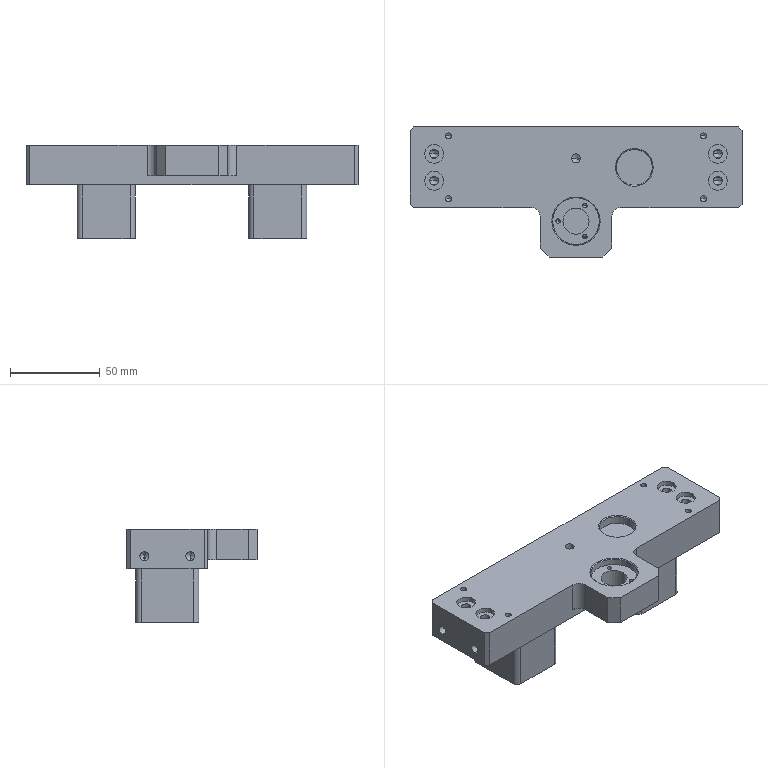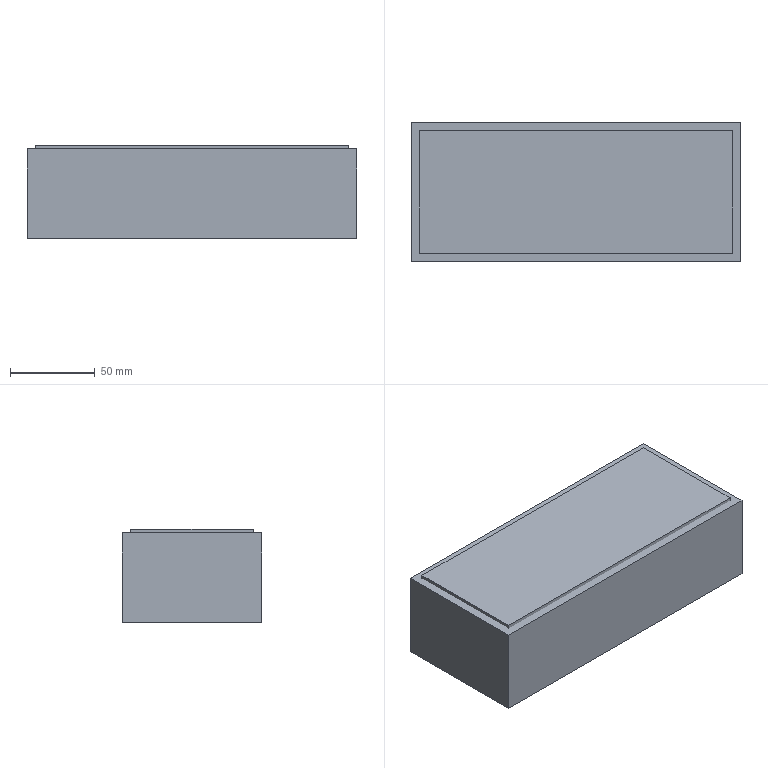CAM job | NX | 3-axis milling, drilling | part box 185 x 72.5 x 52 mm | stock box 195 x 82.5 x 55 mm
Tools:
number,name,description,diameter,corner_radius,flute_length,length,flutes
19,D80,Milling Tool-5 Parameters,80.0,0.0,50.0,75.0,2
1,D6A45,Milling Tool-5 Parameters,6.0,0.0,50.0,75.0,2
4,4.2ZT,Drilling Tool,4.2,0.0,35.0,50.0,2
15,D10,Milling Tool-5 Parameters,10.0,0.0,50.0,75.0,2
14,D10JING,Milling Tool-5 Parameters,10.0,0.0,50.0,75.0,2
3,3.3ZT,Drilling Tool,3.3,0.0,35.0,50.0,2
2,2.5ZT,Drilling Tool,2.5,0.0,35.0,50.0,2
5,5.0ZT,Drilling Tool,5.0,0.0,35.0,50.0,2
12,D6,Milling Tool-5 Parameters,6.0,0.0,50.0,75.0,2
17,D3,Milling Tool-5 Parameters,3.0,0.0,50.0,75.0,2
Operations:
program,operation,operation_type,tool,method,geometry_group,spindle_rpm,surface_speed,feed_per_tooth,feed_cut,feed_plunge,cut_length_mm,path_length_mm,cut_time_min,machine_time_min
1,FLOOR_WALL_COPY,VolumeBased25DMillingOperation,D80,METHOD,A,6500.0,1633.0,0.1154,1500.0,100.0,616.497,670.497,0.411,0.4164
1,DRILLING_COPY_1,Operation,D6A45,METHOD,A,5000.0,94.0,0.035,350.0,0.0,41.6,383.862,0.1189,0.1531
1,DRILLING_COPY_COPY,Operation,4.2ZT,METHOD,A,1516.0,20.0,0.0594,180.0,0.0,331.243,963.147,1.84,1.903
1,CAVITY_MILL,CavityMilling,D10,METHOD,A,9500.0,298.0,0.1316,2500.0,700.0,148448.43,150216.811,59.886,60.063
1,ZLEVEL_PROFILE_COPY_1_COPY_COPY_1,ZLevelMilling,D10JING,METHOD,A,9500.0,298.0,0.0632,1200.0,1000.0,674.661,1186.321,0.5646,0.6158
1,ZLEVEL_PROFILE_COPY_1_COPY_COPY_1_COPY,ZLevelMilling,D10JING,METHOD,A,9500.0,298.0,0.0632,1200.0,1000.0,538.918,700.918,0.4497,0.4659
1,FLOOR_WALL,VolumeBased25DMillingOperation,D10JING,METHOD,A,9500.0,119.0,0.0658,1250.0,100.0,2453.617,4032.575,1.963,2.121
1,PLANAR_MILL_COPY_COPY_COPY_COPY_COPY_COPY_1,PlanarMilling,D6A45,METHOD,A,9500.0,179.0,0.0658,1250.0,100.0,284.431,519.428,0.2275,0.251
1,PLANAR_MILL_COPY_COPY_COPY_COPY_COPY_COPY_1_COPY,PlanarMilling,D6A45,METHOD,A,9500.0,179.0,0.0658,1250.0,100.0,467.645,586.645,0.3741,0.386
1,PLANAR_MILL_COPY_COPY_COPY_COPY_COPY_COPY_1_COPY_COPY,PlanarMilling,D6A45,METHOD,A,9500.0,179.0,0.0658,1250.0,100.0,91.735,220.735,0.0734,0.0863
2,ZLEVEL_PROFILE_1,ZLevelMilling,D10,METHOD,B,9500.0,298.0,0.1316,2500.0,1000.0,1921.309,4071.787,0.7793,0.9943
2,FLOOR_WALL_COPY_COPY,VolumeBased25DMillingOperation,D80,METHOD,B,6500.0,1633.0,0.1154,1500.0,100.0,1759.491,1996.486,1.173,1.197
2,DRILLING_COPY_1_COPY,Operation,D6A45,METHOD,B,5000.0,94.0,0.035,350.0,0.0,56.0,497.398,0.16,0.2041
2,DRILLING_COPY_COPY_1,Operation,3.3ZT,METHOD,B,2000.0,20.0,0.045,180.0,0.0,53.966,389.22,0.2998,0.3333
2,DRILLING_COPY_COPY_1_COPY_1,Operation,3.3ZT,METHOD,B,2000.0,20.0,0.045,180.0,0.0,11.491,82.983,0.0638,0.071
2,DRILLING_COPY_COPY_1_COPY,Operation,2.5ZT,METHOD,B,2006.0,15.0,0.0299,120.0,0.0,45.753,192.663,0.3813,0.396
2,DRILLING_COPY_COPY_COPY,Operation,5.0ZT,METHOD,B,1516.0,20.0,0.0594,180.0,0.0,84.009,425.64,0.4667,0.5009
2,HOLE_MILLING,CylinderMilling,D10,METHOD,B,9500.0,298.0,0.1158,2200.0,100.0,718.842,895.172,0.3267,0.3444
2,HOLE_MILLING_COPY,CylinderMilling,D10,METHOD,B,9500.0,298.0,0.1158,2200.0,100.0,182.136,260.186,0.0828,0.0906
2,HOLE_MILLING_COPY_COPY,CylinderMilling,D6,METHOD,B,9500.0,179.0,0.0868,1650.0,100.0,503.545,938.345,0.3052,0.3487
2,HOLE_MILLING_COPY_COPY_COPY,CylinderMilling,D3,METHOD,B,9500.0,89.0,0.0632,1200.0,100.0,248.964,315.464,0.2075,0.2141
2,FLOOR_WALL_COPY_1,VolumeBased25DMillingOperation,D10JING,METHOD,B,9500.0,119.0,0.0658,1250.0,100.0,106.202,309.319,0.085,0.1053
2,PLANAR_MILL_COPY_COPY_COPY_COPY_COPY_COPY_1_COPY_1,PlanarMilling,D6A45,METHOD,B,9500.0,179.0,0.0658,1250.0,100.0,690.804,1543.66,0.5526,0.6379
2,PLANAR_MILL_COPY_COPY_COPY_COPY_COPY_COPY_1_COPY_1_COPY,PlanarMilling,D6A45,METHOD,B,9500.0,179.0,0.0658,1250.0,100.0,148.419,307.276,0.1187,0.1346
2,刀补,VolumeBased25DMillingOperation,D10JING,METHOD,B,9500.0,119.0,0.0658,1250.0,100.0,59.793,124.893,0.0478,0.0543
2,刀补17,CylinderMilling,D3,METHOD,B,9500.0,89.0,0.0447,850.0,100.0,35.729,102.229,0.042,0.0487